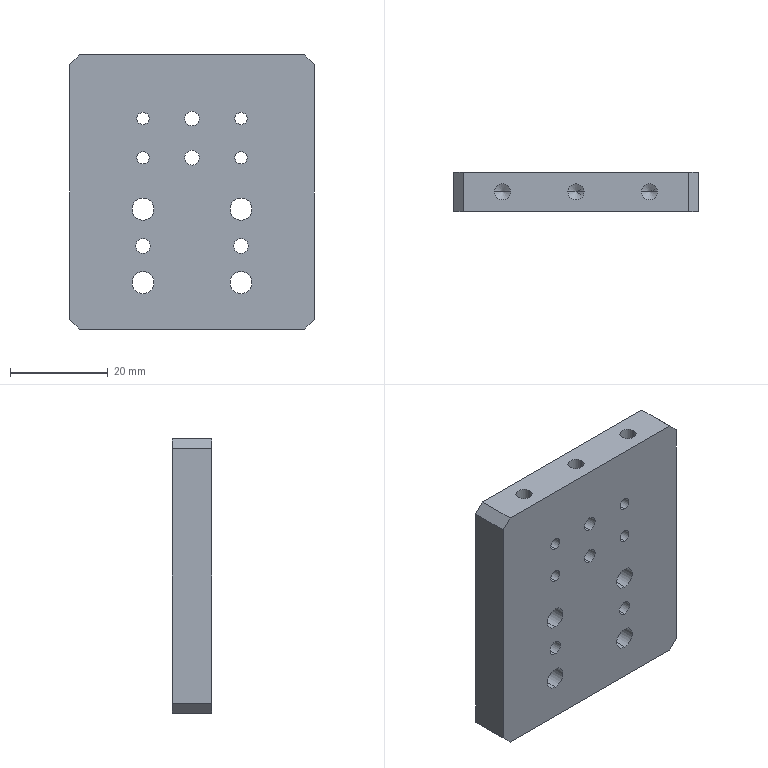Part | SolidWorks | features HoleWzd 8, Chamfer 2, Extrusion 1 | 1 solid | 70 faces | box 50 x 8 x 56 mm | volume 20280 mm3 | cylinder 44 | plane 14 | cone 12 | commonest cylinder face diameters 3.3 x12 2.5 x8 3 x8 4.5 x8 8 x8